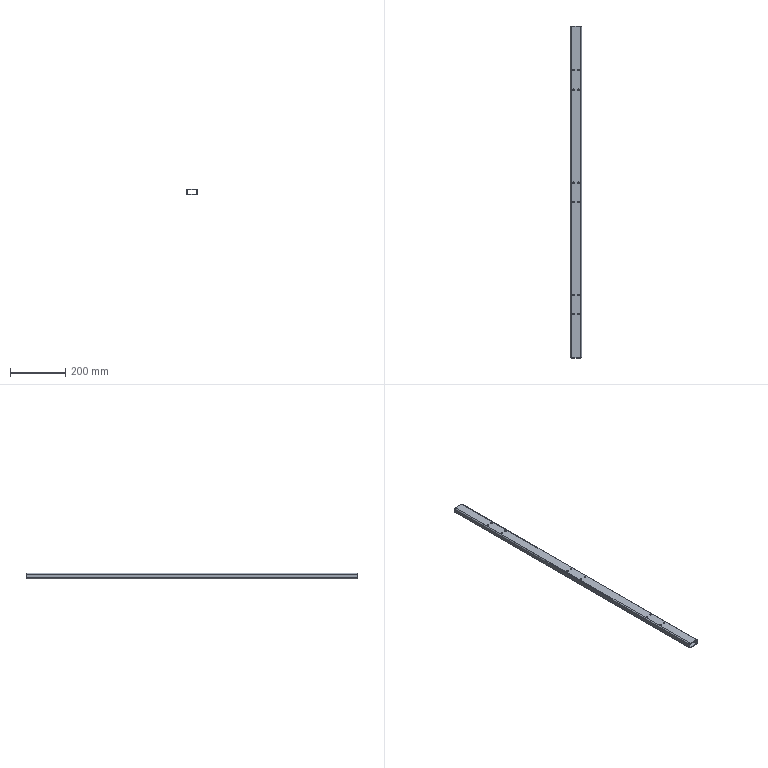Part | SolidWorks | features HoleWzd 1, LPattern 1, WeldMemberFeat 1, WeldmentFeature 1 | 1 solid | 66 faces | box 40 x 1200 x 20 mm | volume 255420 mm3 | cylinder 56 | plane 10 | commonest cylinder face diameters 5.2 x48 4 x4 8 x4